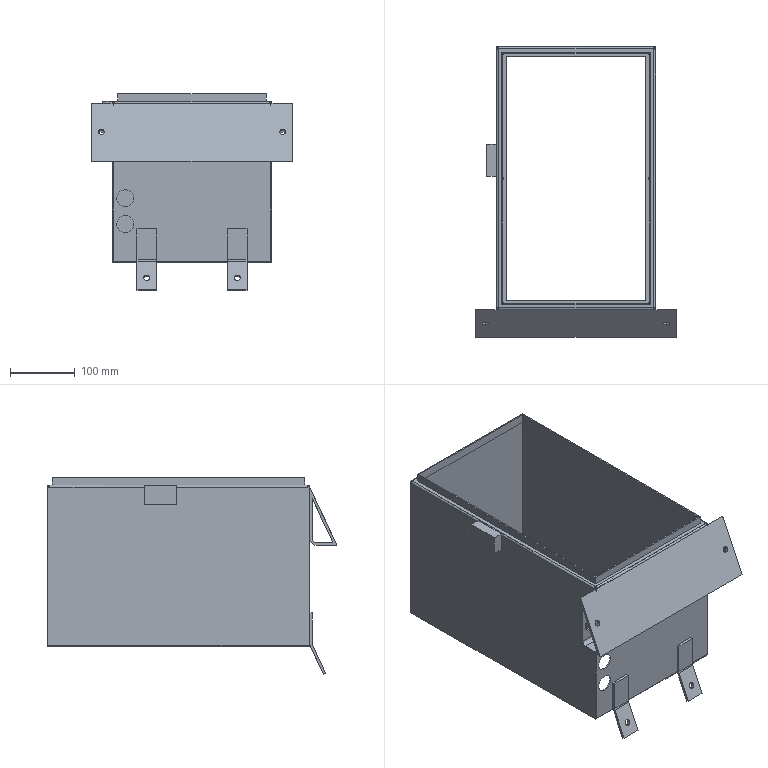Part | STEP file | Cabinet body | 1 solid | 132 faces | box 310 x 447.968 x 304.324 mm | volume 1012965 mm3 | cylinder 54 | plane 54 | spline 24 | commonest cylinder face diameters 3.3 x12 1.473 x8 5.473 x8 9 x8 20 x7 2 x4